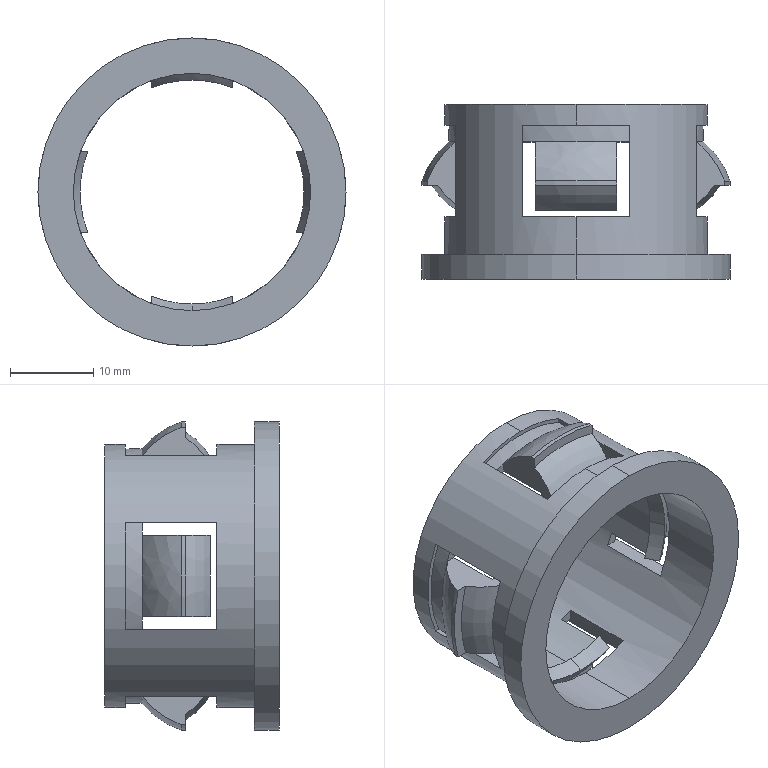Part | STEP file | P2858E25_EINSATZ_VERSCH. | 1 solid | 73 faces | box 37 x 21 x 37 mm | volume 4042 mm3 | plane 43 | cylinder 16 | spline 8 | cone 6 | commonest cylinder face diameters 37 x7 30.6 x5 28.5 x2 31.6 x2